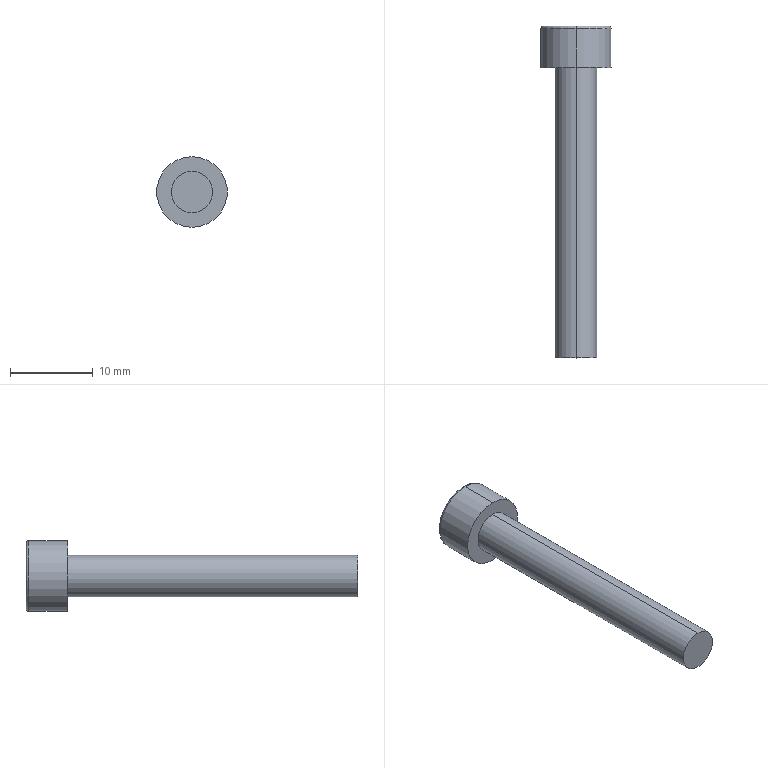Part | STEP file | M5 socket head cap screw simplified_M5X35 | 1 solid | 16 faces | box 8.5 x 40 x 8.5 mm | volume 934.046 mm3 | plane 10 | cylinder 4 | torus 2 | commonest cylinder face diameters 5 x2 8.5 x2
STEP:
#1=CARTESIAN_POINT('',(0.,0.,0.));
#2=DIRECTION('',(0.,0.,1.));
#3=DIRECTION('',(1.,0.,0.));
#4=AXIS2_PLACEMENT_3D('',#1,#2,#3);
#5=CARTESIAN_POINT('',(0.,0.,3.95));
#6=VERTEX_POINT('',#5);
#7=CARTESIAN_POINT('',(0.,0.,-3.95));
#8=VERTEX_POINT('',#7);
#9=CARTESIAN_POINT('',(0.,0.,0.));
#10=DIRECTION('',(0.,1.,0.));
#11=DIRECTION('',(0.,0.,-1.));
#12=AXIS2_PLACEMENT_3D('',#9,#10,#11);
#13=CIRCLE('',#12,3.95);
#14=CARTESIAN_POINT('',(0.,-0.3,0.));
#15=DIRECTION('',(0.,-1.,0.));
#16=DIRECTION('',(0.,0.,-1.));
#17=AXIS2_PLACEMENT_3D('',#14,#15,#16);
#18=TOROIDAL_SURFACE('',#17,3.95,0.3);
#19=CARTESIAN_POINT('',(6.283,4.712));
#20=DIRECTION('',(-1.,0.));
#21=VECTOR('',#20,1.);
#22=LINE('',#19,#21);
#23=(GEOMETRIC_REPRESENTATION_CONTEXT(2)PARAMETRIC_REPRESENTATION_CONTEXT()REPRESENTATION_CONTEXT('',''));
#24=DEFINITIONAL_REPRESENTATION('',(#22),#23);
#25=PCURVE('',#18,#24);
#26=CARTESIAN_POINT('',(0.,0.,0.));
#27=DIRECTION('',(0.,-1.,0.));
#28=DIRECTION('',(0.,0.,-1.));
#29=AXIS2_PLACEMENT_3D('',#26,#27,#28);
#30=PLANE('',#29);
#31=CARTESIAN_POINT('',(3.95,0.));
#32=CARTESIAN_POINT('',(3.95,-6.842));
#33=CARTESIAN_POINT('',(-1.975,-3.421));
#34=CARTESIAN_POINT('',(-7.9,0.));
#35=CARTESIAN_POINT('',(-1.975,3.421));
#36=CARTESIAN_POINT('',(3.95,6.842));
#37=CARTESIAN_POINT('',(3.95,0.));
#38=(BOUNDED_CURVE()B_SPLINE_CURVE(2,(#31,#32,#33,#34,#35,#36,#37),.UNSPECIFIED.,.T.,.F.)B_SPLINE_CURVE_WITH_KNOTS((1,2,2,2,2,1),(-2.094,0.,2.094,4.189,6.283,8.378),.UNSPECIFIED.)CURVE()GEOMETRIC_REPRESENTATION_ITEM()RATIONAL_B_SPLINE_CURVE((1.,0.5,1.,0.5,1.,0.5,1.))REPRESENTATION_ITEM(''));
#39=(GEOMETRIC_REPRESENTATION_CONTEXT(2)PARAMETRIC_REPRESENTATION_CONTEXT()REPRESENTATION_CONTEXT('',''));
#40=DEFINITIONAL_REPRESENTATION('',(#38),#39);
#41=PCURVE('',#30,#40);
#42=SURFACE_CURVE('',#13,(#25,#41),.PCURVE_S1.);
#43=EDGE_CURVE('',#6,#8,#42,.T.);
#44=ORIENTED_EDGE('',*,*,#43,.F.);
#45=CARTESIAN_POINT('',(0.,-0.3,4.25));
#46=VERTEX_POINT('',#45);
#47=CARTESIAN_POINT('',(0.,-0.3,3.95));
#48=DIRECTION('',(1.,0.,0.));
#49=DIRECTION('',(0.,0.,-1.));
#50=AXIS2_PLACEMENT_3D('',#47,#48,#49);
#51=CIRCLE('',#50,0.3);
#52=CARTESIAN_POINT('',(3.142,3.142));
#53=DIRECTION('',(0.,1.));
#54=VECTOR('',#53,1.);
#55=LINE('',#52,#54);
#56=(GEOMETRIC_REPRESENTATION_CONTEXT(2)PARAMETRIC_REPRESENTATION_CONTEXT()REPRESENTATION_CONTEXT('',''));
#57=DEFINITIONAL_REPRESENTATION('',(#55),#56);
#58=PCURVE('',#18,#57);
#59=CARTESIAN_POINT('',(0.,-0.3,0.));
#60=DIRECTION('',(0.,-1.,0.));
#61=DIRECTION('',(0.,0.,-1.));
#62=AXIS2_PLACEMENT_3D('',#59,#60,#61);
#63=TOROIDAL_SURFACE('',#62,3.95,0.3);
#64=CARTESIAN_POINT('',(3.142,3.142));
#65=DIRECTION('',(0.,1.));
#66=VECTOR('',#65,1.);
#67=LINE('',#64,#66);
#68=(GEOMETRIC_REPRESENTATION_CONTEXT(2)PARAMETRIC_REPRESENTATION_CONTEXT()REPRESENTATION_CONTEXT('',''));
#69=DEFINITIONAL_REPRESENTATION('',(#67),#68);
#70=PCURVE('',#63,#69);
#71=SURFACE_CURVE('',#51,(#58,#70),.PCURVE_S1.);
#72=EDGE_CURVE('',#6,#46,#71,.T.);
#73=ORIENTED_EDGE('',*,*,#72,.T.);
#74=CARTESIAN_POINT('',(0.,-0.3,-4.25));
#75=VERTEX_POINT('',#74);
#76=CARTESIAN_POINT('',(0.,-0.3,0.));
#77=DIRECTION('',(0.,-1.,0.));
#78=DIRECTION('',(0.,0.,-1.));
#79=AXIS2_PLACEMENT_3D('',#76,#77,#78);
#80=CIRCLE('',#79,4.25);
#81=CARTESIAN_POINT('',(0.,6.283));
#82=DIRECTION('',(1.,0.));
#83=VECTOR('',#82,1.);
#84=LINE('',#81,#83);
#85=(GEOMETRIC_REPRESENTATION_CONTEXT(2)PARAMETRIC_REPRESENTATION_CONTEXT()REPRESENTATION_CONTEXT('',''));
#86=DEFINITIONAL_REPRESENTATION('',(#84),#85);
#87=PCURVE('',#18,#86);
#88=CARTESIAN_POINT('',(0.,0.,0.));
#89=DIRECTION('',(0.,1.,0.));
#90=DIRECTION('',(0.,0.,1.));
#91=AXIS2_PLACEMENT_3D('',#88,#89,#90);
#92=CYLINDRICAL_SURFACE('',#91,4.25);
#93=CARTESIAN_POINT('',(3.142,-0.3));
#94=DIRECTION('',(-1.,0.));
#95=VECTOR('',#94,1.);
#96=LINE('',#93,#95);
#97=(GEOMETRIC_REPRESENTATION_CONTEXT(2)PARAMETRIC_REPRESENTATION_CONTEXT()REPRESENTATION_CONTEXT('',''));
#98=DEFINITIONAL_REPRESENTATION('',(#96),#97);
#99=PCURVE('',#92,#98);
#100=SURFACE_CURVE('',#80,(#87,#99),.PCURVE_S1.);
#101=EDGE_CURVE('',#75,#46,#100,.T.);
#102=ORIENTED_EDGE('',*,*,#101,.F.);
#103=CARTESIAN_POINT('',(0.,-0.3,-3.95));
#104=DIRECTION('',(-1.,0.,0.));
#105=DIRECTION('',(0.,0.,1.));
#106=AXIS2_PLACEMENT_3D('',#103,#104,#105);
#107=CIRCLE('',#106,0.3);
#108=CARTESIAN_POINT('',(0.,3.142));
#109=DIRECTION('',(0.,1.));
#110=VECTOR('',#109,1.);
#111=LINE('',#108,#110);
#112=(GEOMETRIC_REPRESENTATION_CONTEXT(2)PARAMETRIC_REPRESENTATION_CONTEXT()REPRESENTATION_CONTEXT('',''));
#113=DEFINITIONAL_REPRESENTATION('',(#111),#112);
#114=PCURVE('',#18,#113);
#115=CARTESIAN_POINT('',(6.283,3.142));
#116=DIRECTION('',(0.,1.));
#117=VECTOR('',#116,1.);
#118=LINE('',#115,#117);
#119=(GEOMETRIC_REPRESENTATION_CONTEXT(2)PARAMETRIC_REPRESENTATION_CONTEXT()REPRESENTATION_CONTEXT('',''));
#120=DEFINITIONAL_REPRESENTATION('',(#118),#119);
#121=PCURVE('',#63,#120);
#122=SURFACE_CURVE('',#107,(#114,#121),.PCURVE_S1.);
#123=EDGE_CURVE('',#8,#75,#122,.T.);
#124=ORIENTED_EDGE('',*,*,#123,.F.);
#125=EDGE_LOOP('',(#44,#73,#102,#124));
#126=FACE_BOUND('',#125,.T.);
#127=ADVANCED_FACE('',(#126),#18,.T.);
#128=CARTESIAN_POINT('',(0.,-40.,2.5));
#129=VERTEX_POINT('',#128);
#130=CARTESIAN_POINT('',(0.,-40.,-2.5));
#131=VERTEX_POINT('',#130);
#132=CARTESIAN_POINT('',(0.,-40.,0.));
#133=DIRECTION('',(0.,1.,0.));
#134=DIRECTION('',(0.,0.,1.));
#135=AXIS2_PLACEMENT_3D('',#132,#133,#134);
#136=CIRCLE('',#135,2.5);
#137=CARTESIAN_POINT('',(0.,0.,0.));
#138=DIRECTION('',(0.,1.,0.));
#139=DIRECTION('',(0.,0.,1.));
#140=AXIS2_PLACEMENT_3D('',#137,#138,#139);
#141=CYLINDRICAL_SURFACE('',#140,2.5);
#142=CARTESIAN_POINT('',(0.,-40.));
#143=DIRECTION('',(1.,0.));
#144=VECTOR('',#143,1.);
#145=LINE('',#142,#144);
#146=(GEOMETRIC_REPRESENTATION_CONTEXT(2)PARAMETRIC_REPRESENTATION_CONTEXT()REPRESENTATION_CONTEXT('',''));
#147=DEFINITIONAL_REPRESENTATION('',(#145),#146);
#148=PCURVE('',#141,#147);
#149=CARTESIAN_POINT('',(2.5,-40.,0.));
#150=DIRECTION('',(0.,1.,0.));
#151=DIRECTION('',(0.,0.,1.));
#152=AXIS2_PLACEMENT_3D('',#149,#150,#151);
#153=PLANE('',#152);
#154=CARTESIAN_POINT('',(0.,-2.5));
#155=DIRECTION('',(1.,0.));
#156=AXIS2_PLACEMENT_2D('',#154,#155);
#157=CIRCLE('',#156,2.5);
#158=(GEOMETRIC_REPRESENTATION_CONTEXT(2)PARAMETRIC_REPRESENTATION_CONTEXT()REPRESENTATION_CONTEXT('',''));
#159=DEFINITIONAL_REPRESENTATION('',(#157),#158);
#160=PCURVE('',#153,#159);
#161=SURFACE_CURVE('',#136,(#148,#160),.PCURVE_S1.);
#162=EDGE_CURVE('',#129,#131,#161,.T.);
#163=ORIENTED_EDGE('',*,*,#162,.T.);
#164=CARTESIAN_POINT('',(0.,-5.,-2.5));
#165=VERTEX_POINT('',#164);
#166=CARTESIAN_POINT('',(0.,0.,-2.5));
#167=DIRECTION('',(0.,1.,0.));
#168=VECTOR('',#167,1.);
#169=LINE('',#166,#168);
#170=CARTESIAN_POINT('',(3.142,0.));
#171=DIRECTION('',(0.,1.));
#172=VECTOR('',#171,1.);
#173=LINE('',#170,#172);
#174=(GEOMETRIC_REPRESENTATION_CONTEXT(2)PARAMETRIC_REPRESENTATION_CONTEXT()REPRESENTATION_CONTEXT('',''));
#175=DEFINITIONAL_REPRESENTATION('',(#173),#174);
#176=PCURVE('',#141,#175);
#177=CARTESIAN_POINT('',(0.,0.,0.));
#178=DIRECTION('',(0.,1.,0.));
#179=DIRECTION('',(0.,0.,1.));
#180=AXIS2_PLACEMENT_3D('',#177,#178,#179);
#181=CYLINDRICAL_SURFACE('',#180,2.5);
#182=CARTESIAN_POINT('',(3.142,0.));
#183=DIRECTION('',(0.,1.));
#184=VECTOR('',#183,1.);
#185=LINE('',#182,#184);
#186=(GEOMETRIC_REPRESENTATION_CONTEXT(2)PARAMETRIC_REPRESENTATION_CONTEXT()REPRESENTATION_CONTEXT('',''));
#187=DEFINITIONAL_REPRESENTATION('',(#185),#186);
#188=PCURVE('',#181,#187);
#189=SURFACE_CURVE('',#169,(#176,#188),.PCURVE_S1.);
#190=EDGE_CURVE('',#131,#165,#189,.T.);
#191=ORIENTED_EDGE('',*,*,#190,.T.);
#192=CARTESIAN_POINT('',(0.,-5.,2.5));
#193=VERTEX_POINT('',#192);
#194=CARTESIAN_POINT('',(0.,-5.,0.));
#195=DIRECTION('',(0.,1.,0.));
#196=DIRECTION('',(0.,0.,1.));
#197=AXIS2_PLACEMENT_3D('',#194,#195,#196);
#198=CIRCLE('',#197,2.5);
#199=CARTESIAN_POINT('',(0.,-5.));
#200=DIRECTION('',(1.,0.));
#201=VECTOR('',#200,1.);
#202=LINE('',#199,#201);
#203=(GEOMETRIC_REPRESENTATION_CONTEXT(2)PARAMETRIC_REPRESENTATION_CONTEXT()REPRESENTATION_CONTEXT('',''));
#204=DEFINITIONAL_REPRESENTATION('',(#202),#203);
#205=PCURVE('',#141,#204);
#206=CARTESIAN_POINT('',(4.25,-5.,0.));
#207=DIRECTION('',(0.,1.,0.));
#208=DIRECTION('',(0.,0.,1.));
#209=AXIS2_PLACEMENT_3D('',#206,#207,#208);
#210=PLANE('',#209);
#211=CARTESIAN_POINT('',(0.,-4.25));
#212=DIRECTION('',(1.,0.));
#213=AXIS2_PLACEMENT_2D('',#211,#212);
#214=CIRCLE('',#213,2.5);
#215=(GEOMETRIC_REPRESENTATION_CONTEXT(2)PARAMETRIC_REPRESENTATION_CONTEXT()REPRESENTATION_CONTEXT('',''));
#216=DEFINITIONAL_REPRESENTATION('',(#214),#215);
#217=PCURVE('',#210,#216);
#218=SURFACE_CURVE('',#198,(#205,#217),.PCURVE_S1.);
#219=EDGE_CURVE('',#193,#165,#218,.T.);
#220=ORIENTED_EDGE('',*,*,#219,.F.);
#221=CARTESIAN_POINT('',(0.,0.,2.5));
#222=DIRECTION('',(0.,1.,0.));
#223=VECTOR('',#222,1.);
#224=LINE('',#221,#223);
#225=CARTESIAN_POINT('',(0.,0.));
#226=DIRECTION('',(0.,1.));
#227=VECTOR('',#226,1.);
#228=LINE('',#225,#227);
#229=(GEOMETRIC_REPRESENTATION_CONTEXT(2)PARAMETRIC_REPRESENTATION_CONTEXT()REPRESENTATION_CONTEXT('',''));
#230=DEFINITIONAL_REPRESENTATION('',(#228),#229);
#231=PCURVE('',#141,#230);
#232=CARTESIAN_POINT('',(6.283,0.));
#233=DIRECTION('',(0.,1.));
#234=VECTOR('',#233,1.);
#235=LINE('',#232,#234);
#236=(GEOMETRIC_REPRESENTATION_CONTEXT(2)PARAMETRIC_REPRESENTATION_CONTEXT()REPRESENTATION_CONTEXT('',''));
#237=DEFINITIONAL_REPRESENTATION('',(#235),#236);
#238=PCURVE('',#181,#237);
#239=SURFACE_CURVE('',#224,(#231,#238),.PCURVE_S1.);
#240=EDGE_CURVE('',#129,#193,#239,.T.);
#241=ORIENTED_EDGE('',*,*,#240,.F.);
#242=EDGE_LOOP('',(#163,#191,#220,#241));
#243=FACE_BOUND('',#242,.T.);
#244=ADVANCED_FACE('',(#243),#141,.T.);
#245=CARTESIAN_POINT('',(0.,-5.,4.25));
#246=VERTEX_POINT('',#245);
#247=CARTESIAN_POINT('',(0.,-5.,-4.25));
#248=VERTEX_POINT('',#247);
#249=CARTESIAN_POINT('',(0.,-5.,0.));
#250=DIRECTION('',(0.,1.,0.));
#251=DIRECTION('',(0.,0.,1.));
#252=AXIS2_PLACEMENT_3D('',#249,#250,#251);
#253=CIRCLE('',#252,4.25);
#254=CARTESIAN_POINT('',(0.,-5.));
#255=DIRECTION('',(1.,0.));
#256=VECTOR('',#255,1.);
#257=LINE('',#254,#256);
#258=(GEOMETRIC_REPRESENTATION_CONTEXT(2)PARAMETRIC_REPRESENTATION_CONTEXT()REPRESENTATION_CONTEXT('',''));
#259=DEFINITIONAL_REPRESENTATION('',(#257),#258);
#260=PCURVE('',#92,#259);
#261=CARTESIAN_POINT('',(0.,-4.25));
#262=DIRECTION('',(1.,0.));
#263=AXIS2_PLACEMENT_2D('',#261,#262);
#264=CIRCLE('',#263,4.25);
#265=(GEOMETRIC_REPRESENTATION_CONTEXT(2)PARAMETRIC_REPRESENTATION_CONTEXT()REPRESENTATION_CONTEXT('',''));
#266=DEFINITIONAL_REPRESENTATION('',(#264),#265);
#267=PCURVE('',#210,#266);
#268=SURFACE_CURVE('',#253,(#260,#267),.PCURVE_S1.);
#269=EDGE_CURVE('',#246,#248,#268,.T.);
#270=ORIENTED_EDGE('',*,*,#269,.T.);
#271=CARTESIAN_POINT('',(0.,0.,-4.25));
#272=DIRECTION('',(0.,1.,0.));
#273=VECTOR('',#272,1.);
#274=LINE('',#271,#273);
#275=CARTESIAN_POINT('',(3.142,0.));
#276=DIRECTION('',(0.,1.));
#277=VECTOR('',#276,1.);
#278=LINE('',#275,#277);
#279=(GEOMETRIC_REPRESENTATION_CONTEXT(2)PARAMETRIC_REPRESENTATION_CONTEXT()REPRESENTATION_CONTEXT('',''));
#280=DEFINITIONAL_REPRESENTATION('',(#278),#279);
#281=PCURVE('',#92,#280);
#282=CARTESIAN_POINT('',(0.,0.,0.));
#283=DIRECTION('',(0.,1.,0.));
#284=DIRECTION('',(0.,0.,1.));
#285=AXIS2_PLACEMENT_3D('',#282,#283,#284);
#286=CYLINDRICAL_SURFACE('',#285,4.25);
#287=CARTESIAN_POINT('',(3.142,0.));
#288=DIRECTION('',(0.,1.));
#289=VECTOR('',#288,1.);
#290=LINE('',#287,#289);
#291=(GEOMETRIC_REPRESENTATION_CONTEXT(2)PARAMETRIC_REPRESENTATION_CONTEXT()REPRESENTATION_CONTEXT('',''));
#292=DEFINITIONAL_REPRESENTATION('',(#290),#291);
#293=PCURVE('',#286,#292);
#294=SURFACE_CURVE('',#274,(#281,#293),.PCURVE_S1.);
#295=EDGE_CURVE('',#248,#75,#294,.T.);
#296=ORIENTED_EDGE('',*,*,#295,.T.);
#297=ORIENTED_EDGE('',*,*,#101,.T.);
#298=CARTESIAN_POINT('',(0.,0.,4.25));
#299=DIRECTION('',(0.,1.,0.));
#300=VECTOR('',#299,1.);
#301=LINE('',#298,#300);
#302=CARTESIAN_POINT('',(0.,0.));
#303=DIRECTION('',(0.,1.));
#304=VECTOR('',#303,1.);
#305=LINE('',#302,#304);
#306=(GEOMETRIC_REPRESENTATION_CONTEXT(2)PARAMETRIC_REPRESENTATION_CONTEXT()REPRESENTATION_CONTEXT('',''));
#307=DEFINITIONAL_REPRESENTATION('',(#305),#306);
#308=PCURVE('',#92,#307);
#309=CARTESIAN_POINT('',(6.283,0.));
#310=DIRECTION('',(0.,1.));
#311=VECTOR('',#310,1.);
#312=LINE('',#309,#311);
#313=(GEOMETRIC_REPRESENTATION_CONTEXT(2)PARAMETRIC_REPRESENTATION_CONTEXT()REPRESENTATION_CONTEXT('',''));
#314=DEFINITIONAL_REPRESENTATION('',(#312),#313);
#315=PCURVE('',#286,#314);
#316=SURFACE_CURVE('',#301,(#308,#315),.PCURVE_S1.);
#317=EDGE_CURVE('',#246,#46,#316,.T.);
#318=ORIENTED_EDGE('',*,*,#317,.F.);
#319=EDGE_LOOP('',(#270,#296,#297,#318));
#320=FACE_BOUND('',#319,.T.);
#321=ADVANCED_FACE('',(#320),#92,.T.);
#322=CARTESIAN_POINT('',(0.,0.,0.));
#323=DIRECTION('',(0.,1.,0.));
#324=DIRECTION('',(0.,0.,-1.));
#325=AXIS2_PLACEMENT_3D('',#322,#323,#324);
#326=CIRCLE('',#325,3.95);
#327=CARTESIAN_POINT('',(3.95,0.));
#328=CARTESIAN_POINT('',(3.95,-6.842));
#329=CARTESIAN_POINT('',(-1.975,-3.421));
#330=CARTESIAN_POINT('',(-7.9,0.));
#331=CARTESIAN_POINT('',(-1.975,3.421));
#332=CARTESIAN_POINT('',(3.95,6.842));
#333=CARTESIAN_POINT('',(3.95,0.));
#334=(BOUNDED_CURVE()B_SPLINE_CURVE(2,(#327,#328,#329,#330,#331,#332,#333),.UNSPECIFIED.,.T.,.F.)B_SPLINE_CURVE_WITH_KNOTS((1,2,2,2,2,1),(-2.094,0.,2.094,4.189,6.283,8.378),.UNSPECIFIED.)CURVE()GEOMETRIC_REPRESENTATION_ITEM()RATIONAL_B_SPLINE_CURVE((1.,0.5,1.,0.5,1.,0.5,1.))REPRESENTATION_ITEM(''));
#335=(GEOMETRIC_REPRESENTATION_CONTEXT(2)PARAMETRIC_REPRESENTATION_CONTEXT()REPRESENTATION_CONTEXT('',''));
#336=DEFINITIONAL_REPRESENTATION('',(#334),#335);
#337=PCURVE('',#30,#336);
#338=CARTESIAN_POINT('',(6.283,4.712));
#339=DIRECTION('',(-1.,0.));
#340=VECTOR('',#339,1.);
#341=LINE('',#338,#340);
#342=(GEOMETRIC_REPRESENTATION_CONTEXT(2)PARAMETRIC_REPRESENTATION_CONTEXT()REPRESENTATION_CONTEXT('',''));
#343=DEFINITIONAL_REPRESENTATION('',(#341),#342);
#344=PCURVE('',#63,#343);
#345=SURFACE_CURVE('',#326,(#337,#344),.PCURVE_S1.);
#346=EDGE_CURVE('',#8,#6,#345,.T.);
#347=ORIENTED_EDGE('',*,*,#346,.T.);
#348=ORIENTED_EDGE('',*,*,#43,.T.);
#349=EDGE_LOOP('',(#347,#348));
#350=FACE_BOUND('',#349,.T.);
#351=CARTESIAN_POINT('',(-2.367,0.,0.));
#352=VERTEX_POINT('',#351);
#353=CARTESIAN_POINT('',(-1.184,0.,2.05));
#354=VERTEX_POINT('',#353);
#355=CARTESIAN_POINT('',(-2.367,0.,0.));
#356=DIRECTION('',(0.5,0.,0.866));
#357=VECTOR('',#356,1.);
#358=LINE('',#355,#357);
#359=CARTESIAN_POINT('',(0.,-2.367));
#360=DIRECTION('',(-0.866,0.5));
#361=VECTOR('',#360,1.);
#362=LINE('',#359,#361);
#363=(GEOMETRIC_REPRESENTATION_CONTEXT(2)PARAMETRIC_REPRESENTATION_CONTEXT()REPRESENTATION_CONTEXT('',''));
#364=DEFINITIONAL_REPRESENTATION('',(#362),#363);
#365=PCURVE('',#30,#364);
#366=CARTESIAN_POINT('',(-2.367,-2.5,0.));
#367=DIRECTION('',(-0.866,0.,0.5));
#368=DIRECTION('',(0.5,0.,0.866));
#369=AXIS2_PLACEMENT_3D('',#366,#367,#368);
#370=PLANE('',#369);
#371=CARTESIAN_POINT('',(0.,2.5));
#372=DIRECTION('',(1.,0.));
#373=VECTOR('',#372,1.);
#374=LINE('',#371,#373);
#375=(GEOMETRIC_REPRESENTATION_CONTEXT(2)PARAMETRIC_REPRESENTATION_CONTEXT()REPRESENTATION_CONTEXT('',''));
#376=DEFINITIONAL_REPRESENTATION('',(#374),#375);
#377=PCURVE('',#370,#376);
#378=SURFACE_CURVE('',#358,(#365,#377),.PCURVE_S1.);
#379=EDGE_CURVE('',#352,#354,#378,.T.);
#380=ORIENTED_EDGE('',*,*,#379,.F.);
#381=CARTESIAN_POINT('',(-1.184,0.,-2.05));
#382=VERTEX_POINT('',#381);
#383=CARTESIAN_POINT('',(-1.184,0.,-2.05));
#384=DIRECTION('',(-0.5,0.,0.866));
#385=VECTOR('',#384,1.);
#386=LINE('',#383,#385);
#387=CARTESIAN_POINT('',(2.05,-1.184));
#388=DIRECTION('',(-0.866,-0.5));
#389=VECTOR('',#388,1.);
#390=LINE('',#387,#389);
#391=(GEOMETRIC_REPRESENTATION_CONTEXT(2)PARAMETRIC_REPRESENTATION_CONTEXT()REPRESENTATION_CONTEXT('',''));
#392=DEFINITIONAL_REPRESENTATION('',(#390),#391);
#393=PCURVE('',#30,#392);
#394=CARTESIAN_POINT('',(-1.184,-2.5,-2.05));
#395=DIRECTION('',(-0.866,0.,-0.5));
#396=DIRECTION('',(-0.5,0.,0.866));
#397=AXIS2_PLACEMENT_3D('',#394,#395,#396);
#398=PLANE('',#397);
#399=CARTESIAN_POINT('',(0.,2.5));
#400=DIRECTION('',(1.,0.));
#401=VECTOR('',#400,1.);
#402=LINE('',#399,#401);
#403=(GEOMETRIC_REPRESENTATION_CONTEXT(2)PARAMETRIC_REPRESENTATION_CONTEXT()REPRESENTATION_CONTEXT('',''));
#404=DEFINITIONAL_REPRESENTATION('',(#402),#403);
#405=PCURVE('',#398,#404);
#406=SURFACE_CURVE('',#386,(#393,#405),.PCURVE_S1.);
#407=EDGE_CURVE('',#382,#352,#406,.T.);
#408=ORIENTED_EDGE('',*,*,#407,.F.);
#409=CARTESIAN_POINT('',(1.184,0.,-2.05));
#410=VERTEX_POINT('',#409);
#411=CARTESIAN_POINT('',(1.184,0.,-2.05));
#412=DIRECTION('',(-1.,0.,0.));
#413=VECTOR('',#412,1.);
#414=LINE('',#411,#413);
#415=CARTESIAN_POINT('',(2.05,1.184));
#416=DIRECTION('',(0.,-1.));
#417=VECTOR('',#416,1.);
#418=LINE('',#415,#417);
#419=(GEOMETRIC_REPRESENTATION_CONTEXT(2)PARAMETRIC_REPRESENTATION_CONTEXT()REPRESENTATION_CONTEXT('',''));
#420=DEFINITIONAL_REPRESENTATION('',(#418),#419);
#421=PCURVE('',#30,#420);
#422=CARTESIAN_POINT('',(1.184,-2.5,-2.05));
#423=DIRECTION('',(0.,0.,-1.));
#424=DIRECTION('',(-1.,0.,0.));
#425=AXIS2_PLACEMENT_3D('',#422,#423,#424);
#426=PLANE('',#425);
#427=CARTESIAN_POINT('',(0.,2.5));
#428=DIRECTION('',(1.,0.));
#429=VECTOR('',#428,1.);
#430=LINE('',#427,#429);
#431=(GEOMETRIC_REPRESENTATION_CONTEXT(2)PARAMETRIC_REPRESENTATION_CONTEXT()REPRESENTATION_CONTEXT('',''));
#432=DEFINITIONAL_REPRESENTATION('',(#430),#431);
#433=PCURVE('',#426,#432);
#434=SURFACE_CURVE('',#414,(#421,#433),.PCURVE_S1.);
#435=EDGE_CURVE('',#410,#382,#434,.T.);
#436=ORIENTED_EDGE('',*,*,#435,.F.);
#437=CARTESIAN_POINT('',(2.367,0.,0.));
#438=VERTEX_POINT('',#437);
#439=CARTESIAN_POINT('',(2.367,0.,0.));
#440=DIRECTION('',(-0.5,0.,-0.866));
#441=VECTOR('',#440,1.);
#442=LINE('',#439,#441);
#443=CARTESIAN_POINT('',(0.,2.367));
#444=DIRECTION('',(0.866,-0.5));
#445=VECTOR('',#444,1.);
#446=LINE('',#443,#445);
#447=(GEOMETRIC_REPRESENTATION_CONTEXT(2)PARAMETRIC_REPRESENTATION_CONTEXT()REPRESENTATION_CONTEXT('',''));
#448=DEFINITIONAL_REPRESENTATION('',(#446),#447);
#449=PCURVE('',#30,#448);
#450=CARTESIAN_POINT('',(2.367,-2.5,0.));
#451=DIRECTION('',(0.866,0.,-0.5));
#452=DIRECTION('',(-0.5,0.,-0.866));
#453=AXIS2_PLACEMENT_3D('',#450,#451,#452);
#454=PLANE('',#453);
#455=CARTESIAN_POINT('',(0.,2.5));
#456=DIRECTION('',(1.,0.));
#457=VECTOR('',#456,1.);
#458=LINE('',#455,#457);
#459=(GEOMETRIC_REPRESENTATION_CONTEXT(2)PARAMETRIC_REPRESENTATION_CONTEXT()REPRESENTATION_CONTEXT('',''));
#460=DEFINITIONAL_REPRESENTATION('',(#458),#459);
#461=PCURVE('',#454,#460);
#462=SURFACE_CURVE('',#442,(#449,#461),.PCURVE_S1.);
#463=EDGE_CURVE('',#438,#410,#462,.T.);
#464=ORIENTED_EDGE('',*,*,#463,.F.);
#465=CARTESIAN_POINT('',(1.184,0.,2.05));
#466=VERTEX_POINT('',#465);
#467=CARTESIAN_POINT('',(1.184,0.,2.05));
#468=DIRECTION('',(0.5,0.,-0.866));
#469=VECTOR('',#468,1.);
#470=LINE('',#467,#469);
#471=CARTESIAN_POINT('',(-2.05,1.184));
#472=DIRECTION('',(0.866,0.5));
#473=VECTOR('',#472,1.);
#474=LINE('',#471,#473);
#475=(GEOMETRIC_REPRESENTATION_CONTEXT(2)PARAMETRIC_REPRESENTATION_CONTEXT()REPRESENTATION_CONTEXT('',''));
#476=DEFINITIONAL_REPRESENTATION('',(#474),#475);
#477=PCURVE('',#30,#476);
#478=CARTESIAN_POINT('',(1.184,-2.5,2.05));
#479=DIRECTION('',(0.866,0.,0.5));
#480=DIRECTION('',(0.5,0.,-0.866));
#481=AXIS2_PLACEMENT_3D('',#478,#479,#480);
#482=PLANE('',#481);
#483=CARTESIAN_POINT('',(0.,2.5));
#484=DIRECTION('',(1.,0.));
#485=VECTOR('',#484,1.);
#486=LINE('',#483,#485);
#487=(GEOMETRIC_REPRESENTATION_CONTEXT(2)PARAMETRIC_REPRESENTATION_CONTEXT()REPRESENTATION_CONTEXT('',''));
#488=DEFINITIONAL_REPRESENTATION('',(#486),#487);
#489=PCURVE('',#482,#488);
#490=SURFACE_CURVE('',#470,(#477,#489),.PCURVE_S1.);
#491=EDGE_CURVE('',#466,#438,#490,.T.);
#492=ORIENTED_EDGE('',*,*,#491,.F.);
#493=CARTESIAN_POINT('',(-1.184,0.,2.05));
#494=DIRECTION('',(1.,0.,0.));
#495=VECTOR('',#494,1.);
#496=LINE('',#493,#495);
#497=CARTESIAN_POINT('',(-2.05,-1.184));
#498=DIRECTION('',(0.,1.));
#499=VECTOR('',#498,1.);
#500=LINE('',#497,#499);
#501=(GEOMETRIC_REPRESENTATION_CONTEXT(2)PARAMETRIC_REPRESENTATION_CONTEXT()REPRESENTATION_CONTEXT('',''));
#502=DEFINITIONAL_REPRESENTATION('',(#500),#501);
#503=PCURVE('',#30,#502);
#504=CARTESIAN_POINT('',(-1.184,-2.5,2.05));
#505=DIRECTION('',(0.,0.,1.));
#506=DIRECTION('',(1.,0.,0.));
#507=AXIS2_PLACEMENT_3D('',#504,#505,#506);
#508=PLANE('',#507);
#509=CARTESIAN_POINT('',(0.,2.5));
#510=DIRECTION('',(1.,0.));
#511=VECTOR('',#510,1.);
#512=LINE('',#509,#511);
#513=(GEOMETRIC_REPRESENTATION_CONTEXT(2)PARAMETRIC_REPRESENTATION_CONTEXT()REPRESENTATION_CONTEXT('',''));
#514=DEFINITIONAL_REPRESENTATION('',(#512),#513);
#515=PCURVE('',#508,#514);
#516=SURFACE_CURVE('',#496,(#503,#515),.PCURVE_S1.);
#517=EDGE_CURVE('',#354,#466,#516,.T.);
#518=ORIENTED_EDGE('',*,*,#517,.F.);
#519=EDGE_LOOP('',(#380,#408,#436,#464,#492,#518));
#520=FACE_BOUND('',#519,.T.);
#521=ADVANCED_FACE('',(#350,#520),#30,.F.);
#522=ORIENTED_EDGE('',*,*,#295,.F.);
#523=CARTESIAN_POINT('',(0.,-5.,0.));
#524=DIRECTION('',(0.,1.,0.));
#525=DIRECTION('',(0.,0.,1.));
#526=AXIS2_PLACEMENT_3D('',#523,#524,#525);
#527=CIRCLE('',#526,4.25);
#528=CARTESIAN_POINT('',(0.,-5.));
#529=DIRECTION('',(1.,0.));
#530=VECTOR('',#529,1.);
#531=LINE('',#528,#530);
#532=(GEOMETRIC_REPRESENTATION_CONTEXT(2)PARAMETRIC_REPRESENTATION_CONTEXT()REPRESENTATION_CONTEXT('',''));
#533=DEFINITIONAL_REPRESENTATION('',(#531),#532);
#534=PCURVE('',#286,#533);
#535=CARTESIAN_POINT('',(0.,-4.25));
#536=DIRECTION('',(1.,0.));
#537=AXIS2_PLACEMENT_2D('',#535,#536);
#538=CIRCLE('',#537,4.25);
#539=(GEOMETRIC_REPRESENTATION_CONTEXT(2)PARAMETRIC_REPRESENTATION_CONTEXT()REPRESENTATION_CONTEXT('',''));
#540=DEFINITIONAL_REPRESENTATION('',(#538),#539);
#541=PCURVE('',#210,#540);
#542=SURFACE_CURVE('',#527,(#534,#541),.PCURVE_S1.);
#543=EDGE_CURVE('',#248,#246,#542,.T.);
#544=ORIENTED_EDGE('',*,*,#543,.T.);
#545=ORIENTED_EDGE('',*,*,#317,.T.);
#546=CARTESIAN_POINT('',(0.,-0.3,0.));
#547=DIRECTION('',(0.,-1.,0.));
#548=DIRECTION('',(0.,0.,-1.));
#549=AXIS2_PLACEMENT_3D('',#546,#547,#548);
#550=CIRCLE('',#549,4.25);
#551=CARTESIAN_POINT('',(9.425,-0.3));
#552=DIRECTION('',(-1.,0.));
#553=VECTOR('',#552,1.);
#554=LINE('',#551,#553);
#555=(GEOMETRIC_REPRESENTATION_CONTEXT(2)PARAMETRIC_REPRESENTATION_CONTEXT()REPRESENTATION_CONTEXT('',''));
#556=DEFINITIONAL_REPRESENTATION('',(#554),#555);
#557=PCURVE('',#286,#556);
#558=CARTESIAN_POINT('',(0.,6.283));
#559=DIRECTION('',(1.,0.));
#560=VECTOR('',#559,1.);
#561=LINE('',#558,#560);
#562=(GEOMETRIC_REPRESENTATION_CONTEXT(2)PARAMETRIC_REPRESENTATION_CONTEXT()REPRESENTATION_CONTEXT('',''));
#563=DEFINITIONAL_REPRESENTATION('',(#561),#562);
#564=PCURVE('',#63,#563);
#565=SURFACE_CURVE('',#550,(#557,#564),.PCURVE_S1.);
#566=EDGE_CURVE('',#46,#75,#565,.T.);
#567=ORIENTED_EDGE('',*,*,#566,.T.);
#568=EDGE_LOOP('',(#522,#544,#545,#567));
#569=FACE_BOUND('',#568,.T.);
#570=ADVANCED_FACE('',(#569),#286,.T.);
#571=ORIENTED_EDGE('',*,*,#269,.F.);
#572=ORIENTED_EDGE('',*,*,#543,.F.);
#573=EDGE_LOOP('',(#571,#572));
#574=FACE_BOUND('',#573,.T.);
#575=ORIENTED_EDGE('',*,*,#219,.T.);
#576=CARTESIAN_POINT('',(0.,-5.,0.));
#577=DIRECTION('',(0.,1.,0.));
#578=DIRECTION('',(0.,0.,1.));
#579=AXIS2_PLACEMENT_3D('',#576,#577,#578);
#580=CIRCLE('',#579,2.5);
#581=CARTESIAN_POINT('',(0.,-4.25));
#582=DIRECTION('',(1.,0.));
#583=AXIS2_PLACEMENT_2D('',#581,#582);
#584=CIRCLE('',#583,2.5);
#585=(GEOMETRIC_REPRESENTATION_CONTEXT(2)PARAMETRIC_REPRESENTATION_CONTEXT()REPRESENTATION_CONTEXT('',''));
#586=DEFINITIONAL_REPRESENTATION('',(#584),#585);
#587=PCURVE('',#210,#586);
#588=CARTESIAN_POINT('',(0.,-5.));
#589=DIRECTION('',(1.,0.));
#590=VECTOR('',#589,1.);
#591=LINE('',#588,#590);
#592=(GEOMETRIC_REPRESENTATION_CONTEXT(2)PARAMETRIC_REPRESENTATION_CONTEXT()REPRESENTATION_CONTEXT('',''));
#593=DEFINITIONAL_REPRESENTATION('',(#591),#592);
#594=PCURVE('',#181,#593);
#595=SURFACE_CURVE('',#580,(#587,#594),.PCURVE_S1.);
#596=EDGE_CURVE('',#165,#193,#595,.T.);
#597=ORIENTED_EDGE('',*,*,#596,.T.);
#598=EDGE_LOOP('',(#575,#597));
#599=FACE_BOUND('',#598,.T.);
#600=ADVANCED_FACE('',(#574,#599),#210,.F.);
#601=ORIENTED_EDGE('',*,*,#190,.F.);
#602=CARTESIAN_POINT('',(0.,-40.,0.));
#603=DIRECTION('',(0.,1.,0.));
#604=DIRECTION('',(0.,0.,1.));
#605=AXIS2_PLACEMENT_3D('',#602,#603,#604);
#606=CIRCLE('',#605,2.5);
#607=CARTESIAN_POINT('',(0.,-40.));
#608=DIRECTION('',(1.,0.));
#609=VECTOR('',#608,1.);
#610=LINE('',#607,#609);
#611=(GEOMETRIC_REPRESENTATION_CONTEXT(2)PARAMETRIC_REPRESENTATION_CONTEXT()REPRESENTATION_CONTEXT('',''));
#612=DEFINITIONAL_REPRESENTATION('',(#610),#611);
#613=PCURVE('',#181,#612);
#614=CARTESIAN_POINT('',(0.,-2.5));
#615=DIRECTION('',(1.,0.));
#616=AXIS2_PLACEMENT_2D('',#614,#615);
#617=CIRCLE('',#616,2.5);
#618=(GEOMETRIC_REPRESENTATION_CONTEXT(2)PARAMETRIC_REPRESENTATION_CONTEXT()REPRESENTATION_CONTEXT('',''));
#619=DEFINITIONAL_REPRESENTATION('',(#617),#618);
#620=PCURVE('',#153,#619);
#621=SURFACE_CURVE('',#606,(#613,#620),.PCURVE_S1.);
#622=EDGE_CURVE('',#131,#129,#621,.T.);
#623=ORIENTED_EDGE('',*,*,#622,.T.);
#624=ORIENTED_EDGE('',*,*,#240,.T.);
#625=ORIENTED_EDGE('',*,*,#596,.F.);
#626=EDGE_LOOP('',(#601,#623,#624,#625));
#627=FACE_BOUND('',#626,.T.);
#628=ADVANCED_FACE('',(#627),#181,.T.);
#629=ORIENTED_EDGE('',*,*,#162,.F.);
#630=ORIENTED_EDGE('',*,*,#622,.F.);
#631=EDGE_LOOP('',(#629,#630));
#632=FACE_BOUND('',#631,.T.);
#633=ADVANCED_FACE('',(#632),#153,.F.);
#634=ORIENTED_EDGE('',*,*,#407,.T.);
#635=CARTESIAN_POINT('',(-2.367,-2.5,0.));
#636=VERTEX_POINT('',#635);
#637=CARTESIAN_POINT('',(-2.367,-2.5,0.));
#638=DIRECTION('',(0.,1.,0.));
#639=VECTOR('',#638,1.);
#640=LINE('',#637,#639);
#641=CARTESIAN_POINT('',(2.367,0.));
#642=DIRECTION('',(0.,1.));
#643=VECTOR('',#642,1.);
#644=LINE('',#641,#643);
#645=(GEOMETRIC_REPRESENTATION_CONTEXT(2)PARAMETRIC_REPRESENTATION_CONTEXT()REPRESENTATION_CONTEXT('',''));
#646=DEFINITIONAL_REPRESENTATION('',(#644),#645);
#647=PCURVE('',#398,#646);
#648=CARTESIAN_POINT('',(0.,0.));
#649=DIRECTION('',(0.,1.));
#650=VECTOR('',#649,1.);
#651=LINE('',#648,#650);
#652=(GEOMETRIC_REPRESENTATION_CONTEXT(2)PARAMETRIC_REPRESENTATION_CONTEXT()REPRESENTATION_CONTEXT('',''));
#653=DEFINITIONAL_REPRESENTATION('',(#651),#652);
#654=PCURVE('',#370,#653);
#655=SURFACE_CURVE('',#640,(#647,#654),.PCURVE_S1.);
#656=EDGE_CURVE('',#636,#352,#655,.T.);
#657=ORIENTED_EDGE('',*,*,#656,.F.);
#658=CARTESIAN_POINT('',(-1.184,-2.5,-2.05));
#659=VERTEX_POINT('',#658);
#660=CARTESIAN_POINT('',(-1.184,-2.5,-2.05));
#661=DIRECTION('',(-0.5,0.,0.866));
#662=VECTOR('',#661,1.);
#663=LINE('',#660,#662);
#664=CARTESIAN_POINT('',(0.,0.));
#665=DIRECTION('',(1.,0.));
#666=VECTOR('',#665,1.);
#667=LINE('',#664,#666);
#668=(GEOMETRIC_REPRESENTATION_CONTEXT(2)PARAMETRIC_REPRESENTATION_CONTEXT()REPRESENTATION_CONTEXT('',''));
#669=DEFINITIONAL_REPRESENTATION('',(#667),#668);
#670=PCURVE('',#398,#669);
#671=CARTESIAN_POINT('',(0.,-2.5,-4.1));
#672=DIRECTION('',(0.,-1.,0.));
#673=DIRECTION('',(0.,0.,-1.));
#674=AXIS2_PLACEMENT_3D('',#671,#672,#673);
#675=PLANE('',#674);
#676=CARTESIAN_POINT('',(-2.05,-1.184));
#677=DIRECTION('',(-0.866,-0.5));
#678=VECTOR('',#677,1.);
#679=LINE('',#676,#678);
#680=(GEOMETRIC_REPRESENTATION_CONTEXT(2)PARAMETRIC_REPRESENTATION_CONTEXT()REPRESENTATION_CONTEXT('',''));
#681=DEFINITIONAL_REPRESENTATION('',(#679),#680);
#682=PCURVE('',#675,#681);
#683=SURFACE_CURVE('',#663,(#670,#682),.PCURVE_S1.);
#684=EDGE_CURVE('',#659,#636,#683,.T.);
#685=ORIENTED_EDGE('',*,*,#684,.F.);
#686=CARTESIAN_POINT('',(-1.184,-2.5,-2.05));
#687=DIRECTION('',(0.,1.,0.));
#688=VECTOR('',#687,1.);
#689=LINE('',#686,#688);
#690=CARTESIAN_POINT('',(0.,0.));
#691=DIRECTION('',(0.,1.));
#692=VECTOR('',#691,1.);
#693=LINE('',#690,#692);
#694=(GEOMETRIC_REPRESENTATION_CONTEXT(2)PARAMETRIC_REPRESENTATION_CONTEXT()REPRESENTATION_CONTEXT('',''));
#695=DEFINITIONAL_REPRESENTATION('',(#693),#694);
#696=PCURVE('',#398,#695);
#697=CARTESIAN_POINT('',(2.367,0.));
#698=DIRECTION('',(0.,1.));
#699=VECTOR('',#698,1.);
#700=LINE('',#697,#699);
#701=(GEOMETRIC_REPRESENTATION_CONTEXT(2)PARAMETRIC_REPRESENTATION_CONTEXT()REPRESENTATION_CONTEXT('',''));
#702=DEFINITIONAL_REPRESENTATION('',(#700),#701);
#703=PCURVE('',#426,#702);
#704=SURFACE_CURVE('',#689,(#696,#703),.PCURVE_S1.);
#705=EDGE_CURVE('',#659,#382,#704,.T.);
#706=ORIENTED_EDGE('',*,*,#705,.T.);
#707=EDGE_LOOP('',(#634,#657,#685,#706));
#708=FACE_BOUND('',#707,.T.);
#709=ADVANCED_FACE('',(#708),#398,.F.);
#710=ORIENTED_EDGE('',*,*,#435,.T.);
#711=ORIENTED_EDGE('',*,*,#705,.F.);
#712=CARTESIAN_POINT('',(1.184,-2.5,-2.05));
#713=VERTEX_POINT('',#712);
#714=CARTESIAN_POINT('',(1.184,-2.5,-2.05));
#715=DIRECTION('',(-1.,0.,0.));
#716=VECTOR('',#715,1.);
#717=LINE('',#714,#716);
#718=CARTESIAN_POINT('',(0.,0.));
#719=DIRECTION('',(1.,0.));
#720=VECTOR('',#719,1.);
#721=LINE('',#718,#720);
#722=(GEOMETRIC_REPRESENTATION_CONTEXT(2)PARAMETRIC_REPRESENTATION_CONTEXT()REPRESENTATION_CONTEXT('',''));
#723=DEFINITIONAL_REPRESENTATION('',(#721),#722);
#724=PCURVE('',#426,#723);
#725=CARTESIAN_POINT('',(-2.05,1.184));
#726=DIRECTION('',(0.,-1.));
#727=VECTOR('',#726,1.);
#728=LINE('',#725,#727);
#729=(GEOMETRIC_REPRESENTATION_CONTEXT(2)PARAMETRIC_REPRESENTATION_CONTEXT()REPRESENTATION_CONTEXT('',''));
#730=DEFINITIONAL_REPRESENTATION('',(#728),#729);
#731=PCURVE('',#675,#730);
#732=SURFACE_CURVE('',#717,(#724,#731),.PCURVE_S1.);
#733=EDGE_CURVE('',#713,#659,#732,.T.);
#734=ORIENTED_EDGE('',*,*,#733,.F.);
#735=CARTESIAN_POINT('',(1.184,-2.5,-2.05));
#736=DIRECTION('',(0.,1.,0.));
#737=VECTOR('',#736,1.);
#738=LINE('',#735,#737);
#739=CARTESIAN_POINT('',(0.,0.));
#740=DIRECTION('',(0.,1.));
#741=VECTOR('',#740,1.);
#742=LINE('',#739,#741);
#743=(GEOMETRIC_REPRESENTATION_CONTEXT(2)PARAMETRIC_REPRESENTATION_CONTEXT()REPRESENTATION_CONTEXT('',''));
#744=DEFINITIONAL_REPRESENTATION('',(#742),#743);
#745=PCURVE('',#426,#744);
#746=CARTESIAN_POINT('',(2.367,0.));
#747=DIRECTION('',(0.,1.));
#748=VECTOR('',#747,1.);
#749=LINE('',#746,#748);
#750=(GEOMETRIC_REPRESENTATION_CONTEXT(2)PARAMETRIC_REPRESENTATION_CONTEXT()REPRESENTATION_CONTEXT('',''));
#751=DEFINITIONAL_REPRESENTATION('',(#749),#750);
#752=PCURVE('',#454,#751);
#753=SURFACE_CURVE('',#738,(#745,#752),.PCURVE_S1.);
#754=EDGE_CURVE('',#713,#410,#753,.T.);
#755=ORIENTED_EDGE('',*,*,#754,.T.);
#756=EDGE_LOOP('',(#710,#711,#734,#755));
#757=FACE_BOUND('',#756,.T.);
#758=ADVANCED_FACE('',(#757),#426,.F.);
#759=ORIENTED_EDGE('',*,*,#463,.T.);
#760=ORIENTED_EDGE('',*,*,#754,.F.);
#761=CARTESIAN_POINT('',(2.367,-2.5,0.));
#762=VERTEX_POINT('',#761);
#763=CARTESIAN_POINT('',(2.367,-2.5,0.));
#764=DIRECTION('',(-0.5,0.,-0.866));
#765=VECTOR('',#764,1.);
#766=LINE('',#763,#765);
#767=CARTESIAN_POINT('',(0.,0.));
#768=DIRECTION('',(1.,0.));
#769=VECTOR('',#768,1.);
#770=LINE('',#767,#769);
#771=(GEOMETRIC_REPRESENTATION_CONTEXT(2)PARAMETRIC_REPRESENTATION_CONTEXT()REPRESENTATION_CONTEXT('',''));
#772=DEFINITIONAL_REPRESENTATION('',(#770),#771);
#773=PCURVE('',#454,#772);
#774=CARTESIAN_POINT('',(-4.1,2.367));
#775=DIRECTION('',(0.866,-0.5));
#776=VECTOR('',#775,1.);
#777=LINE('',#774,#776);
#778=(GEOMETRIC_REPRESENTATION_CONTEXT(2)PARAMETRIC_REPRESENTATION_CONTEXT()REPRESENTATION_CONTEXT('',''));
#779=DEFINITIONAL_REPRESENTATION('',(#777),#778);
#780=PCURVE('',#675,#779);
#781=SURFACE_CURVE('',#766,(#773,#780),.PCURVE_S1.);
#782=EDGE_CURVE('',#762,#713,#781,.T.);
#783=ORIENTED_EDGE('',*,*,#782,.F.);
#784=CARTESIAN_POINT('',(2.367,-2.5,0.));
#785=DIRECTION('',(0.,1.,0.));
#786=VECTOR('',#785,1.);
#787=LINE('',#784,#786);
#788=CARTESIAN_POINT('',(0.,0.));
#789=DIRECTION('',(0.,1.));
#790=VECTOR('',#789,1.);
#791=LINE('',#788,#790);
#792=(GEOMETRIC_REPRESENTATION_CONTEXT(2)PARAMETRIC_REPRESENTATION_CONTEXT()REPRESENTATION_CONTEXT('',''));
#793=DEFINITIONAL_REPRESENTATION('',(#791),#792);
#794=PCURVE('',#454,#793);
#795=CARTESIAN_POINT('',(2.367,0.));
#796=DIRECTION('',(0.,1.));
#797=VECTOR('',#796,1.);
#798=LINE('',#795,#797);
#799=(GEOMETRIC_REPRESENTATION_CONTEXT(2)PARAMETRIC_REPRESENTATION_CONTEXT()REPRESENTATION_CONTEXT('',''));
#800=DEFINITIONAL_REPRESENTATION('',(#798),#799);
#801=PCURVE('',#482,#800);
#802=SURFACE_CURVE('',#787,(#794,#801),.PCURVE_S1.);
#803=EDGE_CURVE('',#762,#438,#802,.T.);
#804=ORIENTED_EDGE('',*,*,#803,.T.);
#805=EDGE_LOOP('',(#759,#760,#783,#804));
#806=FACE_BOUND('',#805,.T.);
#807=ADVANCED_FACE('',(#806),#454,.F.);
#808=ORIENTED_EDGE('',*,*,#491,.T.);
#809=ORIENTED_EDGE('',*,*,#803,.F.);
#810=CARTESIAN_POINT('',(1.184,-2.5,2.05));
#811=VERTEX_POINT('',#810);
#812=CARTESIAN_POINT('',(1.184,-2.5,2.05));
#813=DIRECTION('',(0.5,0.,-0.866));
#814=VECTOR('',#813,1.);
#815=LINE('',#812,#814);
#816=CARTESIAN_POINT('',(0.,0.));
#817=DIRECTION('',(1.,0.));
#818=VECTOR('',#817,1.);
#819=LINE('',#816,#818);
#820=(GEOMETRIC_REPRESENTATION_CONTEXT(2)PARAMETRIC_REPRESENTATION_CONTEXT()REPRESENTATION_CONTEXT('',''));
#821=DEFINITIONAL_REPRESENTATION('',(#819),#820);
#822=PCURVE('',#482,#821);
#823=CARTESIAN_POINT('',(-6.15,1.184));
#824=DIRECTION('',(0.866,0.5));
#825=VECTOR('',#824,1.);
#826=LINE('',#823,#825);
#827=(GEOMETRIC_REPRESENTATION_CONTEXT(2)PARAMETRIC_REPRESENTATION_CONTEXT()REPRESENTATION_CONTEXT('',''));
#828=DEFINITIONAL_REPRESENTATION('',(#826),#827);
#829=PCURVE('',#675,#828);
#830=SURFACE_CURVE('',#815,(#822,#829),.PCURVE_S1.);
#831=EDGE_CURVE('',#811,#762,#830,.T.);
#832=ORIENTED_EDGE('',*,*,#831,.F.);
#833=CARTESIAN_POINT('',(1.184,-2.5,2.05));
#834=DIRECTION('',(0.,1.,0.));
#835=VECTOR('',#834,1.);
#836=LINE('',#833,#835);
#837=CARTESIAN_POINT('',(0.,0.));
#838=DIRECTION('',(0.,1.));
#839=VECTOR('',#838,1.);
#840=LINE('',#837,#839);
#841=(GEOMETRIC_REPRESENTATION_CONTEXT(2)PARAMETRIC_REPRESENTATION_CONTEXT()REPRESENTATION_CONTEXT('',''));
#842=DEFINITIONAL_REPRESENTATION('',(#840),#841);
#843=PCURVE('',#482,#842);
#844=CARTESIAN_POINT('',(2.367,0.));
#845=DIRECTION('',(0.,1.));
#846=VECTOR('',#845,1.);
#847=LINE('',#844,#846);
#848=(GEOMETRIC_REPRESENTATION_CONTEXT(2)PARAMETRIC_REPRESENTATION_CONTEXT()REPRESENTATION_CONTEXT('',''));
#849=DEFINITIONAL_REPRESENTATION('',(#847),#848);
#850=PCURVE('',#508,#849);
#851=SURFACE_CURVE('',#836,(#843,#850),.PCURVE_S1.);
#852=EDGE_CURVE('',#811,#466,#851,.T.);
#853=ORIENTED_EDGE('',*,*,#852,.T.);
#854=EDGE_LOOP('',(#808,#809,#832,#853));
#855=FACE_BOUND('',#854,.T.);
#856=ADVANCED_FACE('',(#855),#482,.F.);
#857=ORIENTED_EDGE('',*,*,#517,.T.);
#858=ORIENTED_EDGE('',*,*,#852,.F.);
#859=CARTESIAN_POINT('',(-1.184,-2.5,2.05));
#860=VERTEX_POINT('',#859);
#861=CARTESIAN_POINT('',(-1.184,-2.5,2.05));
#862=DIRECTION('',(1.,0.,0.));
#863=VECTOR('',#862,1.);
#864=LINE('',#861,#863);
#865=CARTESIAN_POINT('',(0.,0.));
#866=DIRECTION('',(1.,0.));
#867=VECTOR('',#866,1.);
#868=LINE('',#865,#867);
#869=(GEOMETRIC_REPRESENTATION_CONTEXT(2)PARAMETRIC_REPRESENTATION_CONTEXT()REPRESENTATION_CONTEXT('',''));
#870=DEFINITIONAL_REPRESENTATION('',(#868),#869);
#871=PCURVE('',#508,#870);
#872=CARTESIAN_POINT('',(-6.15,-1.184));
#873=DIRECTION('',(0.,1.));
#874=VECTOR('',#873,1.);
#875=LINE('',#872,#874);
#876=(GEOMETRIC_REPRESENTATION_CONTEXT(2)PARAMETRIC_REPRESENTATION_CONTEXT()REPRESENTATION_CONTEXT('',''));
#877=DEFINITIONAL_REPRESENTATION('',(#875),#876);
#878=PCURVE('',#675,#877);
#879=SURFACE_CURVE('',#864,(#871,#878),.PCURVE_S1.);
#880=EDGE_CURVE('',#860,#811,#879,.T.);
#881=ORIENTED_EDGE('',*,*,#880,.F.);
#882=CARTESIAN_POINT('',(-1.184,-2.5,2.05));
#883=DIRECTION('',(0.,1.,0.));
#884=VECTOR('',#883,1.);
#885=LINE('',#882,#884);
#886=CARTESIAN_POINT('',(0.,0.));
#887=DIRECTION('',(0.,1.));
#888=VECTOR('',#887,1.);
#889=LINE('',#886,#888);
#890=(GEOMETRIC_REPRESENTATION_CONTEXT(2)PARAMETRIC_REPRESENTATION_CONTEXT()REPRESENTATION_CONTEXT('',''));
#891=DEFINITIONAL_REPRESENTATION('',(#889),#890);
#892=PCURVE('',#508,#891);
#893=CARTESIAN_POINT('',(2.367,0.));
#894=DIRECTION('',(0.,1.));
#895=VECTOR('',#894,1.);
#896=LINE('',#893,#895);
#897=(GEOMETRIC_REPRESENTATION_CONTEXT(2)PARAMETRIC_REPRESENTATION_CONTEXT()REPRESENTATION_CONTEXT('',''));
#898=DEFINITIONAL_REPRESENTATION('',(#896),#897);
#899=PCURVE('',#370,#898);
#900=SURFACE_CURVE('',#885,(#892,#899),.PCURVE_S1.);
#901=EDGE_CURVE('',#860,#354,#900,.T.);
#902=ORIENTED_EDGE('',*,*,#901,.T.);
#903=EDGE_LOOP('',(#857,#858,#881,#902));
#904=FACE_BOUND('',#903,.T.);
#905=ADVANCED_FACE('',(#904),#508,.F.);
#906=ORIENTED_EDGE('',*,*,#379,.T.);
#907=ORIENTED_EDGE('',*,*,#901,.F.);
#908=CARTESIAN_POINT('',(-2.367,-2.5,0.));
#909=DIRECTION('',(0.5,0.,0.866));
#910=VECTOR('',#909,1.);
#911=LINE('',#908,#910);
#912=CARTESIAN_POINT('',(0.,0.));
#913=DIRECTION('',(1.,0.));
#914=VECTOR('',#913,1.);
#915=LINE('',#912,#914);
#916=(GEOMETRIC_REPRESENTATION_CONTEXT(2)PARAMETRIC_REPRESENTATION_CONTEXT()REPRESENTATION_CONTEXT('',''));
#917=DEFINITIONAL_REPRESENTATION('',(#915),#916);
#918=PCURVE('',#370,#917);
#919=CARTESIAN_POINT('',(-4.1,-2.367));
#920=DIRECTION('',(-0.866,0.5));
#921=VECTOR('',#920,1.);
#922=LINE('',#919,#921);
#923=(GEOMETRIC_REPRESENTATION_CONTEXT(2)PARAMETRIC_REPRESENTATION_CONTEXT()REPRESENTATION_CONTEXT('',''));
#924=DEFINITIONAL_REPRESENTATION('',(#922),#923);
#925=PCURVE('',#675,#924);
#926=SURFACE_CURVE('',#911,(#918,#925),.PCURVE_S1.);
#927=EDGE_CURVE('',#636,#860,#926,.T.);
#928=ORIENTED_EDGE('',*,*,#927,.F.);
#929=ORIENTED_EDGE('',*,*,#656,.T.);
#930=EDGE_LOOP('',(#906,#907,#928,#929));
#931=FACE_BOUND('',#930,.T.);
#932=ADVANCED_FACE('',(#931),#370,.F.);
#933=ORIENTED_EDGE('',*,*,#684,.T.);
#934=ORIENTED_EDGE('',*,*,#927,.T.);
#935=ORIENTED_EDGE('',*,*,#880,.T.);
#936=ORIENTED_EDGE('',*,*,#831,.T.);
#937=ORIENTED_EDGE('',*,*,#782,.T.);
#938=ORIENTED_EDGE('',*,*,#733,.T.);
#939=EDGE_LOOP('',(#933,#934,#935,#936,#937,#938));
#940=FACE_BOUND('',#939,.T.);
#941=ADVANCED_FACE('',(#940),#675,.F.);
#942=ORIENTED_EDGE('',*,*,#72,.F.);
#943=ORIENTED_EDGE('',*,*,#346,.F.);
#944=ORIENTED_EDGE('',*,*,#123,.T.);
#945=ORIENTED_EDGE('',*,*,#566,.F.);
#946=EDGE_LOOP('',(#942,#943,#944,#945));
#947=FACE_BOUND('',#946,.T.);
#948=ADVANCED_FACE('',(#947),#63,.T.);
#949=CLOSED_SHELL('',(#127,#244,#321,#521,#570,#600,#628,#633,#709,#758,#807,#856,#905,#932,#941,#948));
#950=MANIFOLD_SOLID_BREP('',#949);
#951=(LENGTH_UNIT()NAMED_UNIT(*)SI_UNIT(.MILLI.,.METRE.));
#952=UNCERTAINTY_MEASURE_WITH_UNIT(LENGTH_MEASURE(0.0000001),#951,'','');
#953=(NAMED_UNIT(*)PLANE_ANGLE_UNIT()SI_UNIT($,.RADIAN.));
#954=(NAMED_UNIT(*)SI_UNIT($,.STERADIAN.)SOLID_ANGLE_UNIT());
#955=(GEOMETRIC_REPRESENTATION_CONTEXT(3)GLOBAL_UNCERTAINTY_ASSIGNED_CONTEXT((#952))GLOBAL_UNIT_ASSIGNED_CONTEXT((#951,#953,#954))REPRESENTATION_CONTEXT('',''));
#956=ADVANCED_BREP_SHAPE_REPRESENTATION('',(#4,#950),#955);